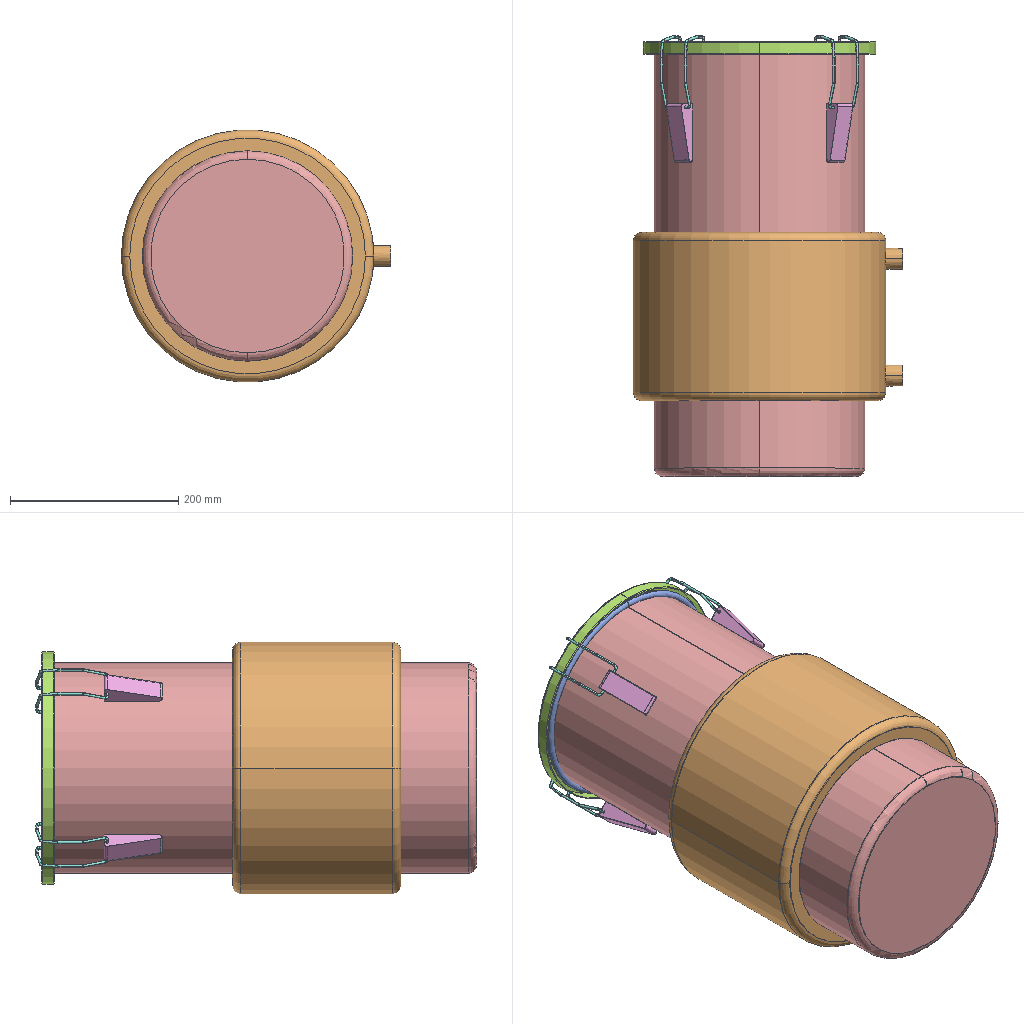Assembly | SolidWorks | 6 different items | 12 placed | box 320 x 524 x 299 mm
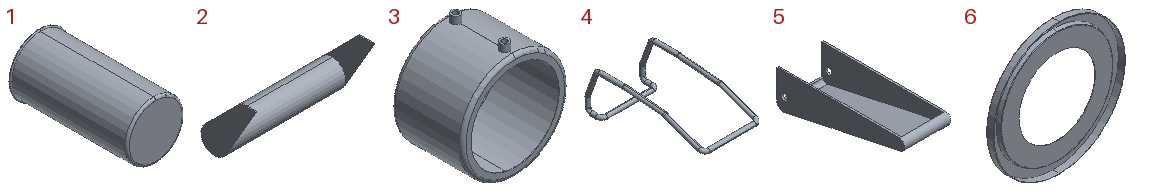Parts list (item | quantity | size | volume | features):
1 | x1 | 264 x 509 x 264 mm | 457801 mm3 | features Extrusion 1, Fillet 1, Revolution 1, Shell 1
2 | x1 | 90 x 41.177 x 44 mm | 6809 mm3 | features Extrusion 1, ICE 1, MirrorPattern 1
3 | x1 | 300 x 200 x 320 mm | 277240 mm3 | features ICE 2, 3DProfileFeature 1, Extrusion 1, Fillet 1, HoleWzd 1, Shell 1
4 | x4 | 43 x 87.917 x 31.794 mm | 2200 mm3 | features 3DProfileFeature 2, MirrorPattern 1, Sweep 1
5 | x4 | 25 x 69.188 x 19.303 mm | 3484 mm3 | features Extrusion 1, Fillet 1, ICE 1, Shell 1
6 | x1 | 276 x 15 x 276 mm | 56604 mm3 | features ICE 2, Fillet 1, Revolution 1
Mates (type | each side: item.copy, entity, surface, feature):
Concentric | 1.1 face cylinder Boss-Extrude1 | 6.1 face cylinder Revolve1
Concentric | 1.1 face cylinder Boss-Extrude1 | 3.1 face cylinder Boss-Extrude1
DistanceDim | 3.1 face plane Boss-Extrude1 | 1.1 face plane Boss-Extrude1
Parallel | 3.1 plane | assembly plane
Concentric | 5.1 face cylinder Cut-Extrude1 | 4.1 face cylinder Sweep1
Symmetric | 5.1 face plane Boss-Extrude1 | 5.1 face plane Boss-Extrude1 | 4.1 plane
Width | 5.1 face plane Boss-Extrude1 | 5.1 face plane Boss-Extrude1 | 1.1 face cylinder Boss-Extrude1
DistanceDim | 5.1 face plane Boss-Extrude1 | 6.1 face plane Cut-Extrude1
Tangent | 1.1 face cylinder Boss-Extrude1 | 5.1 edge